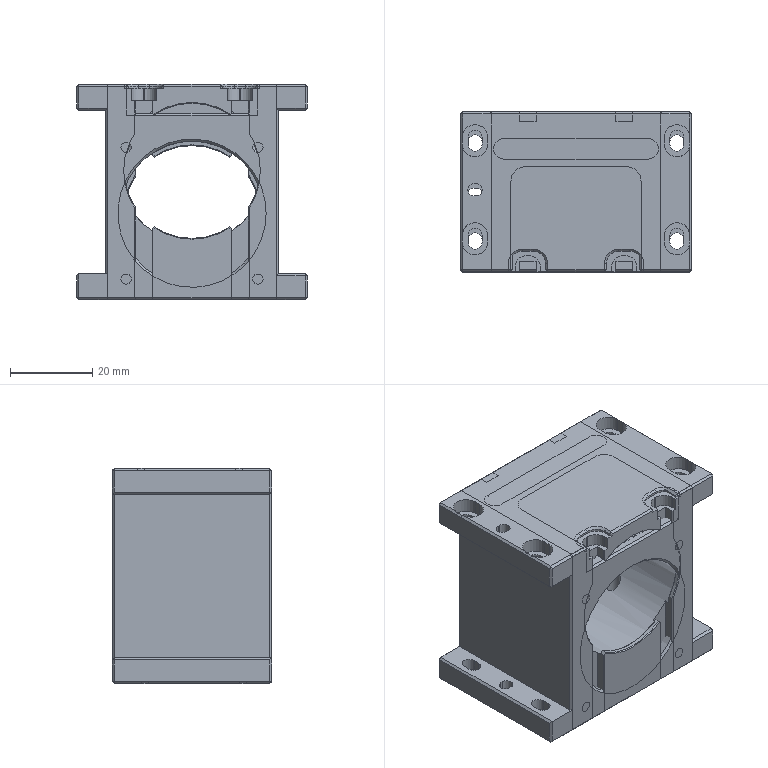CAM job | NX | 3-axis milling, drilling | part box 56 x 38.8 x 52.3 mm | stock box 60 x 45 x 58 mm
Tools:
number,name,description,diameter,corner_radius,flute_length,length,flutes
0,光刀D2.5,,2.5,0.0,7.0,13.0,4
23,光刀D3,,3.0,0.0,8.0,18.2,4
7,光刀D4,Milling Tool-5 Parameters,4.0,0.0,10.0,11.0,4
10,光刀D10,,10.0,0.0,25.0,35.0,4
0,光刀D16,,16.0,0.0,45.0,60.0,4
16,粗刀D3,,3.0,0.0,8.0,18.13,4
7,粗刀D4,Milling Tool-5 Parameters,4.0,0.0,10.0,11.0,4
15,粗刀D10,,10.0,0.0,25.0,40.0,2
0,粗刀D16,,16.0,0.0,40.0,60.0,2
11,倒角刀D6,Chamfer Mill,6.0,0.0,3.0,17.8,2
1,中心钻D6,Spot Drill,6.0,3.0,0.0,17.0,2
5,钻头D2.6,Drilling Tool,2.5,0.0,10.0,30.8,2
4,钻头D3.4,Drilling Tool,3.3,0.0,10.0,25.44,2
2,钻头D5.1,Drilling Tool,5.0,0.0,10.0,40.0,2
20,飞刀D50,,50.0,0.0,50.0,75.0,2
0,ENGRAVER,Milling Tool-5 Parameters,0.1,0.0,2.0,10.0,2
17,M3P0.5螺纹刀单齿柄4,   ,2.4,0.0,0.5,9.809,2
0,M4P0.7螺纹刀单齿柄4,   ,3.2,0.0,0.7,22.608,2
0,M6P1螺纹刀单齿柄6,   ,4.75,0.0,1.0,24.838,4
24,避空刀D2,Milling Tool-5 Parameters,2.0,0.0,5.0,10.0,2
Operations:
program,operation,operation_type,tool,method,geometry_group,spindle_rpm,surface_speed,feed_per_tooth,feed_cut,feed_plunge,cut_length_mm,path_length_mm,cut_time_min,machine_time_min
A-1,飞顶面D50,FaceMilling,飞刀D50,FINISH,WO-1,5500.0,863.938,0.1091,1200.0,100.0,120.0,182.0,0.1,0.1062
A-2,外形动态铣,SurfaceContour,粗刀D16,ROUGHING,WO-1,8500.0,267.035,0.2647,4500.0,1300.0,2455.352,2878.581,0.5165,0.5743
A-2,螺旋内圆D10,CylinderMilling,粗刀D16,SEMI-FINISHING,WO-1,7000.0,351.858,0.1429,2000.0,100.0,3458.744,3599.844,1.729,1.744
A-2,螺旋内圆D10_COPY,CylinderMilling,粗刀D16,SEMI-FINISHING,WO-1,7000.0,351.858,0.1429,2000.0,100.0,336.22,407.12,0.1681,0.1752
A-2,外形动态铣_COPY,SurfaceContour,粗刀D16,ROUGHING,WO-1,8500.0,267.035,0.2647,4500.0,1300.0,2268.469,2342.63,0.4992,0.5103
A-2,外形动态铣_COPY_COPY,SurfaceContour,粗刀D16,ROUGHING,WO-1,8500.0,267.035,0.2647,4500.0,1300.0,2322.982,2397.142,0.5104,0.5215
A-3,轮廓清角-D12,PlanarMilling,粗刀D3,SEMI-FINISHING,WO-1,12000.0,603.186,0.0625,1500.0,100.0,334.396,657.721,0.2229,0.2553
A-3,平面铣螺旋开粗,PlanarMilling,粗刀D3,ROUGHING,WO-1,10000.0,65.973,0.05,1400.0,1300.0,1149.277,1480.677,0.822,0.8658
A-3,轮廓开粗,PlanarMilling,粗刀D3,ROUGHING,WO-1,8500.0,80.111,0.0588,2000.0,100.0,2440.789,2605.119,1.22,1.237
A-4,平面铣螺旋开粗_COPY,PlanarMilling,光刀D2.5,ROUGHING,WO-1,9500.0,119.38,0.0658,2500.0,1300.0,569.34,921.22,0.2336,0.2809
A-4,平面铣螺旋开粗_COPY_COPY,PlanarMilling,光刀D2.5,ROUGHING,WO-1,9500.0,74.613,0.0526,2000.0,1300.0,2245.263,2303.023,1.124,1.132
A-4,单向轮廓精光_COPY_COPY,PlanarMilling,光刀D2.5,光,WO-1,8000.0,251.327,0.0375,600.0,100.0,86.57,453.453,0.1443,0.181
A-5,中心孔M3,Operation,中心钻D6,DRILL,WO-1,2000.0,50.0,0.045,180.0,0.0,2.2,44.4,0.0122,0.0164
A-5,中心孔M3_COPY,Operation,中心钻D6,DRILL,WO-1,2000.0,50.0,0.045,180.0,0.0,8.8,113.423,0.0489,0.0594
A-5,中心孔M3_COPY_COPY,Operation,中心钻D6,DRILL,WO-1,2000.0,50.0,0.045,180.0,0.0,8.8,176.647,0.0489,0.0657
A-6,钻头D3.4-,Operation,钻头D3.4,DRILL,WO-1,2100.0,21.0,0.0595,250.0,0.0,17.34,88.681,0.0694,0.0765
A-7,钻头D5.1-,Operation,钻头D5.1,DRILL,WO-1,1900.0,29.0,0.0658,250.0,0.0,30.486,128.013,0.1219,0.1317
A-8,钻头D2.6-,Operation,钻头D2.6,DRILL,WO-1,2500.0,19.0,0.04,200.0,0.0,9.0,58.0,0.045,0.0499
A-8,钻头D2.6-_COPY,Operation,钻头D2.6,DRILL,WO-1,2500.0,19.0,0.04,200.0,0.0,10.0,74.0,0.05,0.0564
A-8,钻头D2.6-_COPY_COPY,Operation,钻头D2.6,DRILL,WO-1,2500.0,19.0,0.04,200.0,0.0,52.0,256.247,0.26,0.2804
A-9,底壁铣选底,VolumeBased25DMillingOperation,光刀D3,FINISH,WO-1,12000.0,113.097,0.0208,1000.0,100.0,422.236,494.636,0.4222,0.4295
A-9,单向轮廓精光,PlanarMilling,光刀D3,光,WO-1,8000.0,75.398,0.0312,1000.0,100.0,174.594,343.763,0.1746,0.1915
A-9,单向轮廓精光_COPY,PlanarMilling,光刀D3,光,WO-1,8000.0,75.398,0.0312,1000.0,100.0,160.605,500.525,0.1606,0.1946
A-9,单向轮廓精光_COPY_COPY_1,PlanarMilling,光刀D3,光,WO-1,8000.0,75.398,0.0312,1000.0,100.0,158.57,220.57,0.1586,0.1648
A-9,单向轮廓精光_COPY_COPY_1_COPY,PlanarMilling,光刀D3,光,WO-1,8000.0,75.398,0.0312,1000.0,100.0,440.009,699.629,0.44,0.466
A-10,底壁铣选底_1,VolumeBased25DMillingOperation,光刀D10,FINISH,WO-1,9000.0,282.743,0.0333,1200.0,100.0,474.941,568.902,0.3958,0.4052
A-10,单向轮廓精光_1,PlanarMilling,光刀D10,光,WO-1,8000.0,251.327,0.0375,1200.0,100.0,138.968,332.45,0.1158,0.1352
A-10,底壁铣选底_1_COPY,VolumeBased25DMillingOperation,光刀D10,FINISH,WO-1,9000.0,282.743,0.0333,1200.0,100.0,474.941,568.902,0.3958,0.4052
A-10,单向轮廓精光_1_COPY,PlanarMilling,光刀D10,光,WO-1,8000.0,251.327,0.0375,1200.0,100.0,130.684,323.553,0.1089,0.1282
A-10,底壁铣选底_1_COPY_COPY,VolumeBased25DMillingOperation,光刀D10,FINISH,WO-1,9000.0,282.743,0.0333,1200.0,100.0,730.627,815.827,0.6089,0.6174
A-10,底壁铣选底_1_COPY_COPY_COPY,VolumeBased25DMillingOperation,光刀D10,FINISH,WO-1,9000.0,282.743,0.0333,1200.0,100.0,730.627,815.827,0.6089,0.6174
A-10,单向轮廓精光_1_COPY_COPY,PlanarMilling,光刀D10,光,WO-1,8000.0,251.327,0.0375,1200.0,100.0,164.032,222.632,0.1367,0.1426
A-10,单向轮廓精光_1_COPY_COPY_COPY,PlanarMilling,光刀D10,光,WO-1,8000.0,251.327,0.0375,1200.0,100.0,277.936,717.788,0.2316,0.2756
A-10,底壁铣选底_1_COPY_COPY_COPY_COPY,VolumeBased25DMillingOperation,光刀D10,FINISH,WO-1,9000.0,282.743,0.0333,1200.0,100.0,143.884,247.252,0.1199,0.1302
A-10,底壁铣选底_1_COPY_COPY_COPY_COPY_COPY,VolumeBased25DMillingOperation,光刀D10,FINISH,WO-1,9000.0,282.743,0.0333,1200.0,100.0,142.959,246.327,0.1191,0.1295
A-10,底壁铣选底_1_COPY_COPY_COPY_COPY_COPY_COPY,VolumeBased25DMillingOperation,光刀D10,FINISH,WO-1,9000.0,282.743,0.0333,1200.0,100.0,142.954,246.322,0.1191,0.1295
A-10,底壁铣选底_1_COPY_COPY_COPY_COPY_COPY_COPY_COPY,VolumeBased25DMillingOperation,光刀D10,FINISH,WO-1,9000.0,282.743,0.0333,1200.0,100.0,142.89,246.258,0.1191,0.1294
A-10,底壁铣选底_1_COPY_COPY_COPY_COPY_COPY_COPY_COPY_COPY,VolumeBased25DMillingOperation,光刀D10,FINISH,WO-1,9000.0,282.743,0.0333,1200.0,100.0,92.775,165.766,0.0773,0.0846
A-11,倒角刀D6.,PlanarMilling,倒角刀D6,FINISH,WO-1,7500.0,141.372,0.08,1200.0,100.0,98.492,426.492,0.0821,0.1149
A-11,倒角刀D6._COPY,PlanarMilling,倒角刀D6,FINISH,WO-1,7500.0,141.372,0.08,1200.0,100.0,250.777,307.777,0.209,0.2147
A-11,倒角刀D6._COPY_COPY,PlanarMilling,倒角刀D6,FINISH,WO-1,7500.0,141.372,0.08,1200.0,100.0,86.625,143.225,0.0722,0.0778
A-11,倒角刀D6._COPY_COPY_COPY,PlanarMilling,倒角刀D6,FINISH,WO-1,7500.0,141.372,0.02,300.0,100.0,15.111,71.112,0.0504,0.056
A-11,倒角刀D6._COPY_COPY_COPY_COPY,PlanarMilling,倒角刀D6,FINISH,WO-1,7500.0,141.372,0.02,300.0,100.0,14.912,84.311,0.0497,0.0566
A-11,中心孔,Operation,倒角刀D6,DRILL,WO-1,2000.0,50.0,0.045,180.0,0.0,3.1,40.2,0.0172,0.0209
A-11,中心孔_COPY,Operation,倒角刀D6,DRILL,WO-1,2000.0,50.0,0.045,180.0,0.0,8.0,63.042,0.0444,0.0499
A-11,倒角刀D6._COPY_COPY_COPY_COPY_COPY,PlanarMilling,倒角刀D6,FINISH,WO-1,7500.0,141.372,0.02,300.0,100.0,50.1,107.1,0.167,0.1727
A-11,倒角刀D6._COPY_COPY_COPY_COPY_COPY_COPY,PlanarMilling,倒角刀D6,FINISH,WO-1,7500.0,141.372,0.02,300.0,100.0,49.6,106.6,0.1653,0.171
A-11,中心孔_COPY_COPY,Operation,倒角刀D6,DRILL,WO-1,2000.0,50.0,0.045,180.0,0.0,11.2,161.447,0.0622,0.0772
A-11,倒角刀D6._COPY_COPY_COPY_COPY_COPY_COPY_COPY,PlanarMilling,倒角刀D6,FINISH,WO-1,7500.0,141.372,0.02,300.0,100.0,114.382,171.382,0.3813,0.387
A-11,倒角刀D6._COPY_COPY_COPY_COPY_COPY_COPY_COPY_COPY,PlanarMilling,倒角刀D6,FINISH,WO-1,7500.0,141.372,0.02,300.0,100.0,106.216,163.216,0.3541,0.3598
A-11,倒角刀D6._COPY_COPY_COPY_COPY_COPY_COPY_COPY_COPY_COPY,PlanarMilling,倒角刀D6,FINISH,WO-1,7500.0,141.372,0.02,300.0,100.0,224.226,360.026,0.7474,0.761
A-17,曲面区域,SurfaceContour,ENGRAVER,METHOD,WO-1,12000.0,3.77,0.0333,800.0,100.0,127.749,964.601,0.1597,0.2434
A-14,M3螺纹铣,ThreadMilling,M3P0.5螺纹刀单齿柄4,光,WO-1,7000.0,34.086,0.0214,300.0,100.0,260.086,681.756,0.867,0.9091
A-15,M4螺纹铣,ThreadMilling,M4P0.7螺纹刀单齿柄4,光,WO-1,7000.0,70.372,0.0357,500.0,100.0,105.719,206.734,0.2114,0.2215
A-16,M4螺纹铣_COPY,ThreadMilling,M6P1螺纹刀单齿柄6,光,WO-1,7000.0,70.372,0.0357,500.0,100.0,209.73,417.636,0.4195,0.4403
A-12,避空刀精孔.,ZLevelMilling,避空刀D2,FINISH,WO-1,8000.0,50.266,0.0625,1000.0,1000.0,176.185,241.375,0.1762,0.1847
A-12,避空刀精孔._COPY,ZLevelMilling,避空刀D2,FINISH,WO-1,8000.0,50.266,0.0625,1000.0,1000.0,196.615,261.665,0.1966,0.2051
A-12,避空刀精孔._COPY_COPY,ZLevelMilling,避空刀D2,FINISH,WO-1,8000.0,50.266,0.0625,1000.0,1000.0,180.11,259.265,0.1801,0.1904
A-12,避空刀精孔._COPY_COPY_COPY,ZLevelMilling,避空刀D2,FINISH,WO-1,8000.0,50.266,0.0625,1000.0,1000.0,203.057,282.071,0.2031,0.2133
A-13,单向轮廓精光_2,PlanarMilling,光刀D16,光,WO-1,5500.0,251.327,0.0375,800.0,100.0,275.801,404.801,0.3448,0.3577
B-1,外形动态铣_1,SurfaceContour,粗刀D10,ROUGHING,WO-2,8500.0,267.035,0.2647,4500.0,1300.0,1997.518,2046.718,0.4455,0.4529
B-2,轮廓开粗_1_COPY,PlanarMilling,粗刀D4,ROUGHING,WO-2,8000.0,150.796,0.0469,1500.0,100.0,281.97,401.828,0.188,0.2
B-2,轮廓开粗_1,PlanarMilling,粗刀D4,ROUGHING,WO-2,8000.0,150.796,0.0469,1500.0,100.0,89.047,192.263,0.0594,0.0697
B-5,飞顶面D50_1,FaceMilling,飞刀D50,FINISH,WO-2,5500.0,863.938,0.1091,1200.0,100.0,120.0,136.0,0.1,0.1016
B-3,单向轮廓精光_3,PlanarMilling,光刀D4,光,WO-2,8000.0,100.531,0.0219,700.0,100.0,104.505,203.513,0.1493,0.1592
B-3,单向轮廓精光_3_COPY,PlanarMilling,光刀D4,光,WO-2,8000.0,100.531,0.0219,700.0,100.0,72.818,186.458,0.104,0.1154
B-4,倒角刀D6._1,PlanarMilling,倒角刀D6,FINISH,WO-2,7500.0,141.372,0.08,1200.0,100.0,176.024,193.024,0.1467,0.1484
B-4,倒角刀D6._1_COPY,PlanarMilling,倒角刀D6,FINISH,WO-2,7500.0,141.372,0.08,1200.0,100.0,40.57,110.719,0.0338,0.0408
B-4,倒角刀D6._1_COPY_1,PlanarMilling,倒角刀D6,FINISH,WO-2,7500.0,141.372,0.08,1200.0,100.0,52.735,95.448,0.0439,0.0482